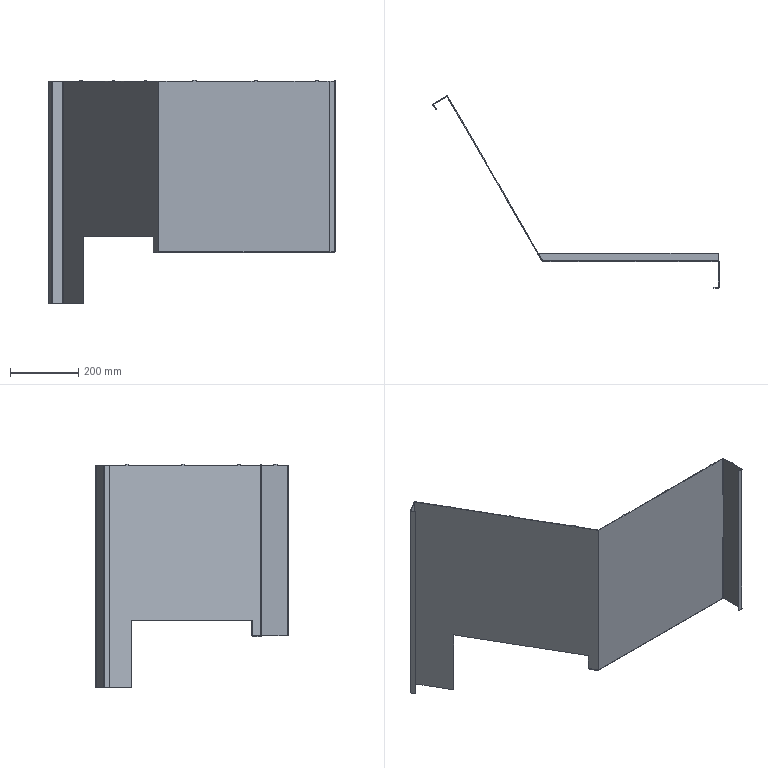Part | STEP file | zq001 | 1 solid | 70 faces | box 840.386 x 564.059 x 655.75 mm | volume 1280382 mm3 | plane 56 | cylinder 14 | commonest cylinder face diameters 1 x7 5 x7